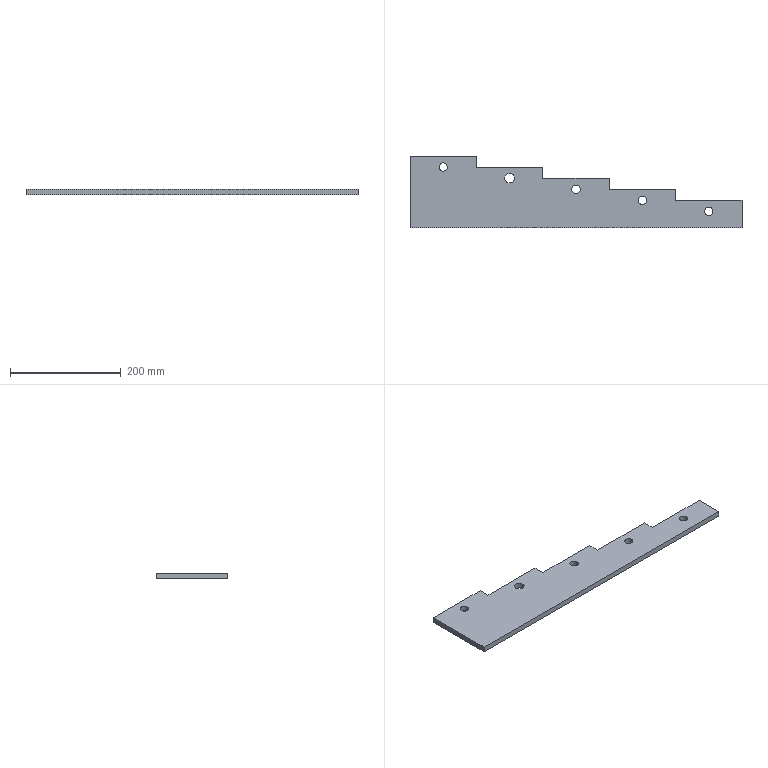Part | SolidWorks | features Extrusion 1 | 1 solid | 24 faces | box 600 x 130 x 10 mm | volume 530579 mm3 | plane 14 | cylinder 10 | commonest cylinder face diameters 15 x8 17.305 x2
STEP:
#1=CARTESIAN_POINT('',(532.5,30.,10.));
#2=VERTEX_POINT('',#1);
#3=CARTESIAN_POINT('',(547.5,30.,10.));
#4=VERTEX_POINT('',#3);
#5=CARTESIAN_POINT('',(540.,30.,10.));
#6=DIRECTION('',(0.,0.,1.));
#7=DIRECTION('',(1.,0.,0.));
#8=AXIS2_PLACEMENT_3D('',#5,#6,#7);
#9=CIRCLE('',#8,7.5);
#10=EDGE_CURVE('',#2,#4,#9,.T.);
#11=ORIENTED_EDGE('',*,*,#10,.T.);
#12=CARTESIAN_POINT('',(547.5,30.,0.));
#13=VERTEX_POINT('',#12);
#14=CARTESIAN_POINT('',(547.5,30.,10.));
#15=DIRECTION('',(0.,0.,-1.));
#16=VECTOR('',#15,1000.);
#17=LINE('',#14,#16);
#18=EDGE_CURVE('',#4,#13,#17,.T.);
#19=ORIENTED_EDGE('',*,*,#18,.T.);
#20=CARTESIAN_POINT('',(532.5,30.,0.));
#21=VERTEX_POINT('',#20);
#22=CARTESIAN_POINT('',(540.,30.,0.));
#23=DIRECTION('',(0.,0.,1.));
#24=DIRECTION('',(1.,0.,0.));
#25=AXIS2_PLACEMENT_3D('',#22,#23,#24);
#26=CIRCLE('',#25,7.5);
#27=EDGE_CURVE('',#21,#13,#26,.T.);
#28=ORIENTED_EDGE('',*,*,#27,.F.);
#29=CARTESIAN_POINT('',(532.5,30.,10.));
#30=DIRECTION('',(0.,0.,-1.));
#31=VECTOR('',#30,1000.);
#32=LINE('',#29,#31);
#33=EDGE_CURVE('',#2,#21,#32,.T.);
#34=ORIENTED_EDGE('',*,*,#33,.F.);
#35=EDGE_LOOP('',(#11,#19,#28,#34));
#36=FACE_OUTER_BOUND('',#35,.T.);
#37=CARTESIAN_POINT('',(540.,30.,10.));
#38=DIRECTION('',(0.,0.,-1.));
#39=DIRECTION('',(-1.,0.,0.));
#40=AXIS2_PLACEMENT_3D('',#37,#38,#39);
#41=CYLINDRICAL_SURFACE('',#40,7.5);
#42=ADVANCED_FACE('',(#36),#41,.F.);
#43=CARTESIAN_POINT('',(412.5,50.,10.));
#44=VERTEX_POINT('',#43);
#45=CARTESIAN_POINT('',(427.5,50.,10.));
#46=VERTEX_POINT('',#45);
#47=CARTESIAN_POINT('',(420.,50.,10.));
#48=DIRECTION('',(0.,0.,1.));
#49=DIRECTION('',(1.,0.,0.));
#50=AXIS2_PLACEMENT_3D('',#47,#48,#49);
#51=CIRCLE('',#50,7.5);
#52=EDGE_CURVE('',#44,#46,#51,.T.);
#53=ORIENTED_EDGE('',*,*,#52,.T.);
#54=CARTESIAN_POINT('',(427.5,50.,0.));
#55=VERTEX_POINT('',#54);
#56=CARTESIAN_POINT('',(427.5,50.,10.));
#57=DIRECTION('',(0.,0.,-1.));
#58=VECTOR('',#57,1000.);
#59=LINE('',#56,#58);
#60=EDGE_CURVE('',#46,#55,#59,.T.);
#61=ORIENTED_EDGE('',*,*,#60,.T.);
#62=CARTESIAN_POINT('',(412.5,50.,0.));
#63=VERTEX_POINT('',#62);
#64=CARTESIAN_POINT('',(420.,50.,0.));
#65=DIRECTION('',(0.,0.,1.));
#66=DIRECTION('',(1.,0.,0.));
#67=AXIS2_PLACEMENT_3D('',#64,#65,#66);
#68=CIRCLE('',#67,7.5);
#69=EDGE_CURVE('',#63,#55,#68,.T.);
#70=ORIENTED_EDGE('',*,*,#69,.F.);
#71=CARTESIAN_POINT('',(412.5,50.,10.));
#72=DIRECTION('',(0.,0.,-1.));
#73=VECTOR('',#72,1000.);
#74=LINE('',#71,#73);
#75=EDGE_CURVE('',#44,#63,#74,.T.);
#76=ORIENTED_EDGE('',*,*,#75,.F.);
#77=EDGE_LOOP('',(#53,#61,#70,#76));
#78=FACE_OUTER_BOUND('',#77,.T.);
#79=CARTESIAN_POINT('',(420.,50.,10.));
#80=DIRECTION('',(0.,0.,-1.));
#81=DIRECTION('',(-1.,0.,0.));
#82=AXIS2_PLACEMENT_3D('',#79,#80,#81);
#83=CYLINDRICAL_SURFACE('',#82,7.5);
#84=ADVANCED_FACE('',(#78),#83,.F.);
#85=CARTESIAN_POINT('',(292.5,70.,10.));
#86=VERTEX_POINT('',#85);
#87=CARTESIAN_POINT('',(307.5,70.,10.));
#88=VERTEX_POINT('',#87);
#89=CARTESIAN_POINT('',(300.,70.,10.));
#90=DIRECTION('',(0.,0.,1.));
#91=DIRECTION('',(1.,0.,0.));
#92=AXIS2_PLACEMENT_3D('',#89,#90,#91);
#93=CIRCLE('',#92,7.5);
#94=EDGE_CURVE('',#86,#88,#93,.T.);
#95=ORIENTED_EDGE('',*,*,#94,.T.);
#96=CARTESIAN_POINT('',(307.5,70.,0.));
#97=VERTEX_POINT('',#96);
#98=CARTESIAN_POINT('',(307.5,70.,10.));
#99=DIRECTION('',(0.,0.,-1.));
#100=VECTOR('',#99,1000.);
#101=LINE('',#98,#100);
#102=EDGE_CURVE('',#88,#97,#101,.T.);
#103=ORIENTED_EDGE('',*,*,#102,.T.);
#104=CARTESIAN_POINT('',(292.5,70.,0.));
#105=VERTEX_POINT('',#104);
#106=CARTESIAN_POINT('',(300.,70.,0.));
#107=DIRECTION('',(0.,0.,1.));
#108=DIRECTION('',(1.,0.,0.));
#109=AXIS2_PLACEMENT_3D('',#106,#107,#108);
#110=CIRCLE('',#109,7.5);
#111=EDGE_CURVE('',#105,#97,#110,.T.);
#112=ORIENTED_EDGE('',*,*,#111,.F.);
#113=CARTESIAN_POINT('',(292.5,70.,10.));
#114=DIRECTION('',(0.,0.,-1.));
#115=VECTOR('',#114,1000.);
#116=LINE('',#113,#115);
#117=EDGE_CURVE('',#86,#105,#116,.T.);
#118=ORIENTED_EDGE('',*,*,#117,.F.);
#119=EDGE_LOOP('',(#95,#103,#112,#118));
#120=FACE_OUTER_BOUND('',#119,.T.);
#121=CARTESIAN_POINT('',(300.,70.,10.));
#122=DIRECTION('',(0.,0.,-1.));
#123=DIRECTION('',(-1.,0.,0.));
#124=AXIS2_PLACEMENT_3D('',#121,#122,#123);
#125=CYLINDRICAL_SURFACE('',#124,7.5);
#126=ADVANCED_FACE('',(#120),#125,.F.);
#127=CARTESIAN_POINT('',(171.348,90.,10.));
#128=VERTEX_POINT('',#127);
#129=CARTESIAN_POINT('',(188.652,90.,10.));
#130=VERTEX_POINT('',#129);
#131=CARTESIAN_POINT('',(180.,90.,10.));
#132=DIRECTION('',(0.,0.,1.));
#133=DIRECTION('',(1.,0.,0.));
#134=AXIS2_PLACEMENT_3D('',#131,#132,#133);
#135=CIRCLE('',#134,8.652);
#136=EDGE_CURVE('',#128,#130,#135,.T.);
#137=ORIENTED_EDGE('',*,*,#136,.T.);
#138=CARTESIAN_POINT('',(188.652,90.,0.));
#139=VERTEX_POINT('',#138);
#140=CARTESIAN_POINT('',(188.652,90.,10.));
#141=DIRECTION('',(0.,0.,-1.));
#142=VECTOR('',#141,1000.);
#143=LINE('',#140,#142);
#144=EDGE_CURVE('',#130,#139,#143,.T.);
#145=ORIENTED_EDGE('',*,*,#144,.T.);
#146=CARTESIAN_POINT('',(171.348,90.,0.));
#147=VERTEX_POINT('',#146);
#148=CARTESIAN_POINT('',(180.,90.,0.));
#149=DIRECTION('',(0.,0.,1.));
#150=DIRECTION('',(1.,0.,0.));
#151=AXIS2_PLACEMENT_3D('',#148,#149,#150);
#152=CIRCLE('',#151,8.652);
#153=EDGE_CURVE('',#147,#139,#152,.T.);
#154=ORIENTED_EDGE('',*,*,#153,.F.);
#155=CARTESIAN_POINT('',(171.348,90.,10.));
#156=DIRECTION('',(0.,0.,-1.));
#157=VECTOR('',#156,1000.);
#158=LINE('',#155,#157);
#159=EDGE_CURVE('',#128,#147,#158,.T.);
#160=ORIENTED_EDGE('',*,*,#159,.F.);
#161=EDGE_LOOP('',(#137,#145,#154,#160));
#162=FACE_OUTER_BOUND('',#161,.T.);
#163=CARTESIAN_POINT('',(180.,90.,10.));
#164=DIRECTION('',(0.,0.,-1.));
#165=DIRECTION('',(-1.,0.,0.));
#166=AXIS2_PLACEMENT_3D('',#163,#164,#165);
#167=CYLINDRICAL_SURFACE('',#166,8.652);
#168=ADVANCED_FACE('',(#162),#167,.F.);
#169=CARTESIAN_POINT('',(52.5,110.,10.));
#170=VERTEX_POINT('',#169);
#171=CARTESIAN_POINT('',(67.5,110.,10.));
#172=VERTEX_POINT('',#171);
#173=CARTESIAN_POINT('',(60.,110.,10.));
#174=DIRECTION('',(0.,0.,1.));
#175=DIRECTION('',(1.,0.,0.));
#176=AXIS2_PLACEMENT_3D('',#173,#174,#175);
#177=CIRCLE('',#176,7.5);
#178=EDGE_CURVE('',#170,#172,#177,.T.);
#179=ORIENTED_EDGE('',*,*,#178,.T.);
#180=CARTESIAN_POINT('',(67.5,110.,0.));
#181=VERTEX_POINT('',#180);
#182=CARTESIAN_POINT('',(67.5,110.,10.));
#183=DIRECTION('',(0.,0.,-1.));
#184=VECTOR('',#183,1000.);
#185=LINE('',#182,#184);
#186=EDGE_CURVE('',#172,#181,#185,.T.);
#187=ORIENTED_EDGE('',*,*,#186,.T.);
#188=CARTESIAN_POINT('',(52.5,110.,0.));
#189=VERTEX_POINT('',#188);
#190=CARTESIAN_POINT('',(60.,110.,0.));
#191=DIRECTION('',(0.,0.,1.));
#192=DIRECTION('',(1.,0.,0.));
#193=AXIS2_PLACEMENT_3D('',#190,#191,#192);
#194=CIRCLE('',#193,7.5);
#195=EDGE_CURVE('',#189,#181,#194,.T.);
#196=ORIENTED_EDGE('',*,*,#195,.F.);
#197=CARTESIAN_POINT('',(52.5,110.,10.));
#198=DIRECTION('',(0.,0.,-1.));
#199=VECTOR('',#198,1000.);
#200=LINE('',#197,#199);
#201=EDGE_CURVE('',#170,#189,#200,.T.);
#202=ORIENTED_EDGE('',*,*,#201,.F.);
#203=EDGE_LOOP('',(#179,#187,#196,#202));
#204=FACE_OUTER_BOUND('',#203,.T.);
#205=CARTESIAN_POINT('',(60.,110.,10.));
#206=DIRECTION('',(0.,0.,-1.));
#207=DIRECTION('',(-1.,0.,0.));
#208=AXIS2_PLACEMENT_3D('',#205,#206,#207);
#209=CYLINDRICAL_SURFACE('',#208,7.5);
#210=ADVANCED_FACE('',(#204),#209,.F.);
#211=ORIENTED_EDGE('',*,*,#52,.F.);
#212=CARTESIAN_POINT('',(420.,50.,10.));
#213=DIRECTION('',(0.,0.,1.));
#214=DIRECTION('',(1.,0.,0.));
#215=AXIS2_PLACEMENT_3D('',#212,#213,#214);
#216=CIRCLE('',#215,7.5);
#217=EDGE_CURVE('',#46,#44,#216,.T.);
#218=ORIENTED_EDGE('',*,*,#217,.F.);
#219=EDGE_LOOP('',(#211,#218));
#220=FACE_BOUND('',#219,.T.);
#221=ORIENTED_EDGE('',*,*,#136,.F.);
#222=CARTESIAN_POINT('',(180.,90.,10.));
#223=DIRECTION('',(0.,0.,1.));
#224=DIRECTION('',(1.,0.,0.));
#225=AXIS2_PLACEMENT_3D('',#222,#223,#224);
#226=CIRCLE('',#225,8.652);
#227=EDGE_CURVE('',#130,#128,#226,.T.);
#228=ORIENTED_EDGE('',*,*,#227,.F.);
#229=EDGE_LOOP('',(#221,#228));
#230=FACE_BOUND('',#229,.T.);
#231=CARTESIAN_POINT('',(0.,130.,10.));
#232=VERTEX_POINT('',#231);
#233=CARTESIAN_POINT('',(0.,0.,10.));
#234=VERTEX_POINT('',#233);
#235=CARTESIAN_POINT('',(0.,130.,10.));
#236=DIRECTION('',(0.,-1.,0.));
#237=VECTOR('',#236,1000.);
#238=LINE('',#235,#237);
#239=EDGE_CURVE('',#232,#234,#238,.T.);
#240=ORIENTED_EDGE('',*,*,#239,.T.);
#241=CARTESIAN_POINT('',(600.,0.,10.));
#242=VERTEX_POINT('',#241);
#243=CARTESIAN_POINT('',(0.,0.,10.));
#244=DIRECTION('',(1.,0.,0.));
#245=VECTOR('',#244,1000.);
#246=LINE('',#243,#245);
#247=EDGE_CURVE('',#234,#242,#246,.T.);
#248=ORIENTED_EDGE('',*,*,#247,.T.);
#249=CARTESIAN_POINT('',(600.,50.,10.));
#250=VERTEX_POINT('',#249);
#251=CARTESIAN_POINT('',(600.,0.,10.));
#252=DIRECTION('',(0.,1.,0.));
#253=VECTOR('',#252,1000.);
#254=LINE('',#251,#253);
#255=EDGE_CURVE('',#242,#250,#254,.T.);
#256=ORIENTED_EDGE('',*,*,#255,.T.);
#257=CARTESIAN_POINT('',(480.,50.,10.));
#258=VERTEX_POINT('',#257);
#259=CARTESIAN_POINT('',(600.,50.,10.));
#260=DIRECTION('',(-1.,0.,0.));
#261=VECTOR('',#260,1000.);
#262=LINE('',#259,#261);
#263=EDGE_CURVE('',#250,#258,#262,.T.);
#264=ORIENTED_EDGE('',*,*,#263,.T.);
#265=CARTESIAN_POINT('',(480.,70.,10.));
#266=VERTEX_POINT('',#265);
#267=CARTESIAN_POINT('',(480.,50.,10.));
#268=DIRECTION('',(0.,1.,0.));
#269=VECTOR('',#268,1000.);
#270=LINE('',#267,#269);
#271=EDGE_CURVE('',#258,#266,#270,.T.);
#272=ORIENTED_EDGE('',*,*,#271,.T.);
#273=CARTESIAN_POINT('',(360.,70.,10.));
#274=VERTEX_POINT('',#273);
#275=CARTESIAN_POINT('',(480.,70.,10.));
#276=DIRECTION('',(-1.,0.,0.));
#277=VECTOR('',#276,1000.);
#278=LINE('',#275,#277);
#279=EDGE_CURVE('',#266,#274,#278,.T.);
#280=ORIENTED_EDGE('',*,*,#279,.T.);
#281=CARTESIAN_POINT('',(360.,90.,10.));
#282=VERTEX_POINT('',#281);
#283=CARTESIAN_POINT('',(360.,70.,10.));
#284=DIRECTION('',(0.,1.,0.));
#285=VECTOR('',#284,1000.);
#286=LINE('',#283,#285);
#287=EDGE_CURVE('',#274,#282,#286,.T.);
#288=ORIENTED_EDGE('',*,*,#287,.T.);
#289=CARTESIAN_POINT('',(240.,90.,10.));
#290=VERTEX_POINT('',#289);
#291=CARTESIAN_POINT('',(360.,90.,10.));
#292=DIRECTION('',(-1.,0.,0.));
#293=VECTOR('',#292,1000.);
#294=LINE('',#291,#293);
#295=EDGE_CURVE('',#282,#290,#294,.T.);
#296=ORIENTED_EDGE('',*,*,#295,.T.);
#297=CARTESIAN_POINT('',(240.,110.,10.));
#298=VERTEX_POINT('',#297);
#299=CARTESIAN_POINT('',(240.,90.,10.));
#300=DIRECTION('',(0.,1.,0.));
#301=VECTOR('',#300,1000.);
#302=LINE('',#299,#301);
#303=EDGE_CURVE('',#290,#298,#302,.T.);
#304=ORIENTED_EDGE('',*,*,#303,.T.);
#305=CARTESIAN_POINT('',(120.,110.,10.));
#306=VERTEX_POINT('',#305);
#307=CARTESIAN_POINT('',(240.,110.,10.));
#308=DIRECTION('',(-1.,0.,0.));
#309=VECTOR('',#308,1000.);
#310=LINE('',#307,#309);
#311=EDGE_CURVE('',#298,#306,#310,.T.);
#312=ORIENTED_EDGE('',*,*,#311,.T.);
#313=CARTESIAN_POINT('',(120.,130.,10.));
#314=VERTEX_POINT('',#313);
#315=CARTESIAN_POINT('',(120.,110.,10.));
#316=DIRECTION('',(0.,1.,0.));
#317=VECTOR('',#316,1000.);
#318=LINE('',#315,#317);
#319=EDGE_CURVE('',#306,#314,#318,.T.);
#320=ORIENTED_EDGE('',*,*,#319,.T.);
#321=CARTESIAN_POINT('',(120.,130.,10.));
#322=DIRECTION('',(-1.,0.,0.));
#323=VECTOR('',#322,1000.);
#324=LINE('',#321,#323);
#325=EDGE_CURVE('',#314,#232,#324,.T.);
#326=ORIENTED_EDGE('',*,*,#325,.T.);
#327=EDGE_LOOP('',(#240,#248,#256,#264,#272,#280,#288,#296,#304,#312,#320,#326));
#328=FACE_OUTER_BOUND('',#327,.T.);
#329=ORIENTED_EDGE('',*,*,#178,.F.);
#330=CARTESIAN_POINT('',(60.,110.,10.));
#331=DIRECTION('',(0.,0.,1.));
#332=DIRECTION('',(1.,0.,0.));
#333=AXIS2_PLACEMENT_3D('',#330,#331,#332);
#334=CIRCLE('',#333,7.5);
#335=EDGE_CURVE('',#172,#170,#334,.T.);
#336=ORIENTED_EDGE('',*,*,#335,.F.);
#337=EDGE_LOOP('',(#329,#336));
#338=FACE_BOUND('',#337,.T.);
#339=ORIENTED_EDGE('',*,*,#94,.F.);
#340=CARTESIAN_POINT('',(300.,70.,10.));
#341=DIRECTION('',(0.,0.,1.));
#342=DIRECTION('',(1.,0.,0.));
#343=AXIS2_PLACEMENT_3D('',#340,#341,#342);
#344=CIRCLE('',#343,7.5);
#345=EDGE_CURVE('',#88,#86,#344,.T.);
#346=ORIENTED_EDGE('',*,*,#345,.F.);
#347=EDGE_LOOP('',(#339,#346));
#348=FACE_BOUND('',#347,.T.);
#349=ORIENTED_EDGE('',*,*,#10,.F.);
#350=CARTESIAN_POINT('',(540.,30.,10.));
#351=DIRECTION('',(0.,0.,1.));
#352=DIRECTION('',(1.,0.,0.));
#353=AXIS2_PLACEMENT_3D('',#350,#351,#352);
#354=CIRCLE('',#353,7.5);
#355=EDGE_CURVE('',#4,#2,#354,.T.);
#356=ORIENTED_EDGE('',*,*,#355,.F.);
#357=EDGE_LOOP('',(#349,#356));
#358=FACE_BOUND('',#357,.T.);
#359=CARTESIAN_POINT('',(0.,0.,10.));
#360=DIRECTION('',(0.,0.,1.));
#361=DIRECTION('',(1.,0.,0.));
#362=AXIS2_PLACEMENT_3D('',#359,#360,#361);
#363=PLANE('',#362);
#364=ADVANCED_FACE('',(#220,#230,#328,#338,#348,#358),#363,.T.);
#365=CARTESIAN_POINT('',(0.,130.,0.));
#366=VERTEX_POINT('',#365);
#367=CARTESIAN_POINT('',(0.,0.,0.));
#368=VERTEX_POINT('',#367);
#369=CARTESIAN_POINT('',(0.,130.,0.));
#370=DIRECTION('',(0.,-1.,0.));
#371=VECTOR('',#370,1000.);
#372=LINE('',#369,#371);
#373=EDGE_CURVE('',#366,#368,#372,.T.);
#374=ORIENTED_EDGE('',*,*,#373,.F.);
#375=CARTESIAN_POINT('',(120.,130.,0.));
#376=VERTEX_POINT('',#375);
#377=CARTESIAN_POINT('',(120.,130.,0.));
#378=DIRECTION('',(-1.,0.,0.));
#379=VECTOR('',#378,1000.);
#380=LINE('',#377,#379);
#381=EDGE_CURVE('',#376,#366,#380,.T.);
#382=ORIENTED_EDGE('',*,*,#381,.F.);
#383=CARTESIAN_POINT('',(120.,110.,0.));
#384=VERTEX_POINT('',#383);
#385=CARTESIAN_POINT('',(120.,110.,0.));
#386=DIRECTION('',(0.,1.,0.));
#387=VECTOR('',#386,1000.);
#388=LINE('',#385,#387);
#389=EDGE_CURVE('',#384,#376,#388,.T.);
#390=ORIENTED_EDGE('',*,*,#389,.F.);
#391=CARTESIAN_POINT('',(240.,110.,0.));
#392=VERTEX_POINT('',#391);
#393=CARTESIAN_POINT('',(240.,110.,0.));
#394=DIRECTION('',(-1.,0.,0.));
#395=VECTOR('',#394,1000.);
#396=LINE('',#393,#395);
#397=EDGE_CURVE('',#392,#384,#396,.T.);
#398=ORIENTED_EDGE('',*,*,#397,.F.);
#399=CARTESIAN_POINT('',(240.,90.,0.));
#400=VERTEX_POINT('',#399);
#401=CARTESIAN_POINT('',(240.,90.,0.));
#402=DIRECTION('',(0.,1.,0.));
#403=VECTOR('',#402,1000.);
#404=LINE('',#401,#403);
#405=EDGE_CURVE('',#400,#392,#404,.T.);
#406=ORIENTED_EDGE('',*,*,#405,.F.);
#407=CARTESIAN_POINT('',(360.,90.,0.));
#408=VERTEX_POINT('',#407);
#409=CARTESIAN_POINT('',(360.,90.,0.));
#410=DIRECTION('',(-1.,0.,0.));
#411=VECTOR('',#410,1000.);
#412=LINE('',#409,#411);
#413=EDGE_CURVE('',#408,#400,#412,.T.);
#414=ORIENTED_EDGE('',*,*,#413,.F.);
#415=CARTESIAN_POINT('',(360.,70.,0.));
#416=VERTEX_POINT('',#415);
#417=CARTESIAN_POINT('',(360.,70.,0.));
#418=DIRECTION('',(0.,1.,0.));
#419=VECTOR('',#418,1000.);
#420=LINE('',#417,#419);
#421=EDGE_CURVE('',#416,#408,#420,.T.);
#422=ORIENTED_EDGE('',*,*,#421,.F.);
#423=CARTESIAN_POINT('',(480.,70.,0.));
#424=VERTEX_POINT('',#423);
#425=CARTESIAN_POINT('',(480.,70.,0.));
#426=DIRECTION('',(-1.,0.,0.));
#427=VECTOR('',#426,1000.);
#428=LINE('',#425,#427);
#429=EDGE_CURVE('',#424,#416,#428,.T.);
#430=ORIENTED_EDGE('',*,*,#429,.F.);
#431=CARTESIAN_POINT('',(480.,50.,0.));
#432=VERTEX_POINT('',#431);
#433=CARTESIAN_POINT('',(480.,50.,0.));
#434=DIRECTION('',(0.,1.,0.));
#435=VECTOR('',#434,1000.);
#436=LINE('',#433,#435);
#437=EDGE_CURVE('',#432,#424,#436,.T.);
#438=ORIENTED_EDGE('',*,*,#437,.F.);
#439=CARTESIAN_POINT('',(600.,50.,0.));
#440=VERTEX_POINT('',#439);
#441=CARTESIAN_POINT('',(600.,50.,0.));
#442=DIRECTION('',(-1.,0.,0.));
#443=VECTOR('',#442,1000.);
#444=LINE('',#441,#443);
#445=EDGE_CURVE('',#440,#432,#444,.T.);
#446=ORIENTED_EDGE('',*,*,#445,.F.);
#447=CARTESIAN_POINT('',(600.,0.,0.));
#448=VERTEX_POINT('',#447);
#449=CARTESIAN_POINT('',(600.,0.,0.));
#450=DIRECTION('',(0.,1.,0.));
#451=VECTOR('',#450,1000.);
#452=LINE('',#449,#451);
#453=EDGE_CURVE('',#448,#440,#452,.T.);
#454=ORIENTED_EDGE('',*,*,#453,.F.);
#455=CARTESIAN_POINT('',(0.,0.,0.));
#456=DIRECTION('',(1.,0.,0.));
#457=VECTOR('',#456,1000.);
#458=LINE('',#455,#457);
#459=EDGE_CURVE('',#368,#448,#458,.T.);
#460=ORIENTED_EDGE('',*,*,#459,.F.);
#461=EDGE_LOOP('',(#374,#382,#390,#398,#406,#414,#422,#430,#438,#446,#454,#460));
#462=FACE_OUTER_BOUND('',#461,.T.);
#463=ORIENTED_EDGE('',*,*,#195,.T.);
#464=CARTESIAN_POINT('',(60.,110.,0.));
#465=DIRECTION('',(0.,0.,1.));
#466=DIRECTION('',(1.,0.,0.));
#467=AXIS2_PLACEMENT_3D('',#464,#465,#466);
#468=CIRCLE('',#467,7.5);
#469=EDGE_CURVE('',#181,#189,#468,.T.);
#470=ORIENTED_EDGE('',*,*,#469,.T.);
#471=EDGE_LOOP('',(#463,#470));
#472=FACE_BOUND('',#471,.T.);
#473=ORIENTED_EDGE('',*,*,#153,.T.);
#474=CARTESIAN_POINT('',(180.,90.,0.));
#475=DIRECTION('',(0.,0.,1.));
#476=DIRECTION('',(1.,0.,0.));
#477=AXIS2_PLACEMENT_3D('',#474,#475,#476);
#478=CIRCLE('',#477,8.652);
#479=EDGE_CURVE('',#139,#147,#478,.T.);
#480=ORIENTED_EDGE('',*,*,#479,.T.);
#481=EDGE_LOOP('',(#473,#480));
#482=FACE_BOUND('',#481,.T.);
#483=ORIENTED_EDGE('',*,*,#111,.T.);
#484=CARTESIAN_POINT('',(300.,70.,0.));
#485=DIRECTION('',(0.,0.,1.));
#486=DIRECTION('',(1.,0.,0.));
#487=AXIS2_PLACEMENT_3D('',#484,#485,#486);
#488=CIRCLE('',#487,7.5);
#489=EDGE_CURVE('',#97,#105,#488,.T.);
#490=ORIENTED_EDGE('',*,*,#489,.T.);
#491=EDGE_LOOP('',(#483,#490));
#492=FACE_BOUND('',#491,.T.);
#493=ORIENTED_EDGE('',*,*,#69,.T.);
#494=CARTESIAN_POINT('',(420.,50.,0.));
#495=DIRECTION('',(0.,0.,1.));
#496=DIRECTION('',(1.,0.,0.));
#497=AXIS2_PLACEMENT_3D('',#494,#495,#496);
#498=CIRCLE('',#497,7.5);
#499=EDGE_CURVE('',#55,#63,#498,.T.);
#500=ORIENTED_EDGE('',*,*,#499,.T.);
#501=EDGE_LOOP('',(#493,#500));
#502=FACE_BOUND('',#501,.T.);
#503=ORIENTED_EDGE('',*,*,#27,.T.);
#504=CARTESIAN_POINT('',(540.,30.,0.));
#505=DIRECTION('',(0.,0.,1.));
#506=DIRECTION('',(1.,0.,0.));
#507=AXIS2_PLACEMENT_3D('',#504,#505,#506);
#508=CIRCLE('',#507,7.5);
#509=EDGE_CURVE('',#13,#21,#508,.T.);
#510=ORIENTED_EDGE('',*,*,#509,.T.);
#511=EDGE_LOOP('',(#503,#510));
#512=FACE_BOUND('',#511,.T.);
#513=CARTESIAN_POINT('',(0.,0.,0.));
#514=DIRECTION('',(0.,0.,1.));
#515=DIRECTION('',(1.,0.,0.));
#516=AXIS2_PLACEMENT_3D('',#513,#514,#515);
#517=PLANE('',#516);
#518=ADVANCED_FACE('',(#462,#472,#482,#492,#502,#512),#517,.F.);
#519=ORIENTED_EDGE('',*,*,#373,.T.);
#520=CARTESIAN_POINT('',(0.,0.,10.));
#521=DIRECTION('',(0.,0.,-1.));
#522=VECTOR('',#521,1000.);
#523=LINE('',#520,#522);
#524=EDGE_CURVE('',#234,#368,#523,.T.);
#525=ORIENTED_EDGE('',*,*,#524,.F.);
#526=ORIENTED_EDGE('',*,*,#239,.F.);
#527=CARTESIAN_POINT('',(0.,130.,10.));
#528=DIRECTION('',(0.,0.,-1.));
#529=VECTOR('',#528,1000.);
#530=LINE('',#527,#529);
#531=EDGE_CURVE('',#232,#366,#530,.T.);
#532=ORIENTED_EDGE('',*,*,#531,.T.);
#533=EDGE_LOOP('',(#519,#525,#526,#532));
#534=FACE_OUTER_BOUND('',#533,.T.);
#535=CARTESIAN_POINT('',(0.,130.,10.));
#536=DIRECTION('',(1.,0.,0.));
#537=DIRECTION('',(0.,0.,-1.));
#538=AXIS2_PLACEMENT_3D('',#535,#536,#537);
#539=PLANE('',#538);
#540=ADVANCED_FACE('',(#534),#539,.F.);
#541=ORIENTED_EDGE('',*,*,#459,.T.);
#542=CARTESIAN_POINT('',(600.,0.,10.));
#543=DIRECTION('',(0.,0.,-1.));
#544=VECTOR('',#543,1000.);
#545=LINE('',#542,#544);
#546=EDGE_CURVE('',#242,#448,#545,.T.);
#547=ORIENTED_EDGE('',*,*,#546,.F.);
#548=ORIENTED_EDGE('',*,*,#247,.F.);
#549=ORIENTED_EDGE('',*,*,#524,.T.);
#550=EDGE_LOOP('',(#541,#547,#548,#549));
#551=FACE_OUTER_BOUND('',#550,.T.);
#552=CARTESIAN_POINT('',(0.,0.,10.));
#553=DIRECTION('',(0.,1.,0.));
#554=DIRECTION('',(0.,0.,1.));
#555=AXIS2_PLACEMENT_3D('',#552,#553,#554);
#556=PLANE('',#555);
#557=ADVANCED_FACE('',(#551),#556,.F.);
#558=ORIENTED_EDGE('',*,*,#453,.T.);
#559=CARTESIAN_POINT('',(600.,50.,10.));
#560=DIRECTION('',(0.,0.,-1.));
#561=VECTOR('',#560,1000.);
#562=LINE('',#559,#561);
#563=EDGE_CURVE('',#250,#440,#562,.T.);
#564=ORIENTED_EDGE('',*,*,#563,.F.);
#565=ORIENTED_EDGE('',*,*,#255,.F.);
#566=ORIENTED_EDGE('',*,*,#546,.T.);
#567=EDGE_LOOP('',(#558,#564,#565,#566));
#568=FACE_OUTER_BOUND('',#567,.T.);
#569=CARTESIAN_POINT('',(600.,0.,10.));
#570=DIRECTION('',(-1.,0.,0.));
#571=DIRECTION('',(0.,0.,1.));
#572=AXIS2_PLACEMENT_3D('',#569,#570,#571);
#573=PLANE('',#572);
#574=ADVANCED_FACE('',(#568),#573,.F.);
#575=ORIENTED_EDGE('',*,*,#445,.T.);
#576=CARTESIAN_POINT('',(480.,50.,10.));
#577=DIRECTION('',(0.,0.,-1.));
#578=VECTOR('',#577,1000.);
#579=LINE('',#576,#578);
#580=EDGE_CURVE('',#258,#432,#579,.T.);
#581=ORIENTED_EDGE('',*,*,#580,.F.);
#582=ORIENTED_EDGE('',*,*,#263,.F.);
#583=ORIENTED_EDGE('',*,*,#563,.T.);
#584=EDGE_LOOP('',(#575,#581,#582,#583));
#585=FACE_OUTER_BOUND('',#584,.T.);
#586=CARTESIAN_POINT('',(600.,50.,10.));
#587=DIRECTION('',(0.,-1.,0.));
#588=DIRECTION('',(1.,0.,0.));
#589=AXIS2_PLACEMENT_3D('',#586,#587,#588);
#590=PLANE('',#589);
#591=ADVANCED_FACE('',(#585),#590,.F.);
#592=ORIENTED_EDGE('',*,*,#437,.T.);
#593=CARTESIAN_POINT('',(480.,70.,10.));
#594=DIRECTION('',(0.,0.,-1.));
#595=VECTOR('',#594,1000.);
#596=LINE('',#593,#595);
#597=EDGE_CURVE('',#266,#424,#596,.T.);
#598=ORIENTED_EDGE('',*,*,#597,.F.);
#599=ORIENTED_EDGE('',*,*,#271,.F.);
#600=ORIENTED_EDGE('',*,*,#580,.T.);
#601=EDGE_LOOP('',(#592,#598,#599,#600));
#602=FACE_OUTER_BOUND('',#601,.T.);
#603=CARTESIAN_POINT('',(480.,50.,10.));
#604=DIRECTION('',(-1.,0.,0.));
#605=DIRECTION('',(0.,0.,1.));
#606=AXIS2_PLACEMENT_3D('',#603,#604,#605);
#607=PLANE('',#606);
#608=ADVANCED_FACE('',(#602),#607,.F.);
#609=ORIENTED_EDGE('',*,*,#429,.T.);
#610=CARTESIAN_POINT('',(360.,70.,10.));
#611=DIRECTION('',(0.,0.,-1.));
#612=VECTOR('',#611,1000.);
#613=LINE('',#610,#612);
#614=EDGE_CURVE('',#274,#416,#613,.T.);
#615=ORIENTED_EDGE('',*,*,#614,.F.);
#616=ORIENTED_EDGE('',*,*,#279,.F.);
#617=ORIENTED_EDGE('',*,*,#597,.T.);
#618=EDGE_LOOP('',(#609,#615,#616,#617));
#619=FACE_OUTER_BOUND('',#618,.T.);
#620=CARTESIAN_POINT('',(480.,70.,10.));
#621=DIRECTION('',(0.,-1.,0.));
#622=DIRECTION('',(1.,0.,0.));
#623=AXIS2_PLACEMENT_3D('',#620,#621,#622);
#624=PLANE('',#623);
#625=ADVANCED_FACE('',(#619),#624,.F.);
#626=ORIENTED_EDGE('',*,*,#421,.T.);
#627=CARTESIAN_POINT('',(360.,90.,10.));
#628=DIRECTION('',(0.,0.,-1.));
#629=VECTOR('',#628,1000.);
#630=LINE('',#627,#629);
#631=EDGE_CURVE('',#282,#408,#630,.T.);
#632=ORIENTED_EDGE('',*,*,#631,.F.);
#633=ORIENTED_EDGE('',*,*,#287,.F.);
#634=ORIENTED_EDGE('',*,*,#614,.T.);
#635=EDGE_LOOP('',(#626,#632,#633,#634));
#636=FACE_OUTER_BOUND('',#635,.T.);
#637=CARTESIAN_POINT('',(360.,70.,10.));
#638=DIRECTION('',(-1.,0.,0.));
#639=DIRECTION('',(0.,0.,1.));
#640=AXIS2_PLACEMENT_3D('',#637,#638,#639);
#641=PLANE('',#640);
#642=ADVANCED_FACE('',(#636),#641,.F.);
#643=ORIENTED_EDGE('',*,*,#413,.T.);
#644=CARTESIAN_POINT('',(240.,90.,10.));
#645=DIRECTION('',(0.,0.,-1.));
#646=VECTOR('',#645,1000.);
#647=LINE('',#644,#646);
#648=EDGE_CURVE('',#290,#400,#647,.T.);
#649=ORIENTED_EDGE('',*,*,#648,.F.);
#650=ORIENTED_EDGE('',*,*,#295,.F.);
#651=ORIENTED_EDGE('',*,*,#631,.T.);
#652=EDGE_LOOP('',(#643,#649,#650,#651));
#653=FACE_OUTER_BOUND('',#652,.T.);
#654=CARTESIAN_POINT('',(360.,90.,10.));
#655=DIRECTION('',(0.,-1.,0.));
#656=DIRECTION('',(1.,0.,0.));
#657=AXIS2_PLACEMENT_3D('',#654,#655,#656);
#658=PLANE('',#657);
#659=ADVANCED_FACE('',(#653),#658,.F.);
#660=ORIENTED_EDGE('',*,*,#405,.T.);
#661=CARTESIAN_POINT('',(240.,110.,10.));
#662=DIRECTION('',(0.,0.,-1.));
#663=VECTOR('',#662,1000.);
#664=LINE('',#661,#663);
#665=EDGE_CURVE('',#298,#392,#664,.T.);
#666=ORIENTED_EDGE('',*,*,#665,.F.);
#667=ORIENTED_EDGE('',*,*,#303,.F.);
#668=ORIENTED_EDGE('',*,*,#648,.T.);
#669=EDGE_LOOP('',(#660,#666,#667,#668));
#670=FACE_OUTER_BOUND('',#669,.T.);
#671=CARTESIAN_POINT('',(240.,90.,10.));
#672=DIRECTION('',(-1.,0.,0.));
#673=DIRECTION('',(0.,0.,1.));
#674=AXIS2_PLACEMENT_3D('',#671,#672,#673);
#675=PLANE('',#674);
#676=ADVANCED_FACE('',(#670),#675,.F.);
#677=ORIENTED_EDGE('',*,*,#397,.T.);
#678=CARTESIAN_POINT('',(120.,110.,10.));
#679=DIRECTION('',(0.,0.,-1.));
#680=VECTOR('',#679,1000.);
#681=LINE('',#678,#680);
#682=EDGE_CURVE('',#306,#384,#681,.T.);
#683=ORIENTED_EDGE('',*,*,#682,.F.);
#684=ORIENTED_EDGE('',*,*,#311,.F.);
#685=ORIENTED_EDGE('',*,*,#665,.T.);
#686=EDGE_LOOP('',(#677,#683,#684,#685));
#687=FACE_OUTER_BOUND('',#686,.T.);
#688=CARTESIAN_POINT('',(240.,110.,10.));
#689=DIRECTION('',(0.,-1.,0.));
#690=DIRECTION('',(1.,0.,0.));
#691=AXIS2_PLACEMENT_3D('',#688,#689,#690);
#692=PLANE('',#691);
#693=ADVANCED_FACE('',(#687),#692,.F.);
#694=ORIENTED_EDGE('',*,*,#389,.T.);
#695=CARTESIAN_POINT('',(120.,130.,10.));
#696=DIRECTION('',(0.,0.,-1.));
#697=VECTOR('',#696,1000.);
#698=LINE('',#695,#697);
#699=EDGE_CURVE('',#314,#376,#698,.T.);
#700=ORIENTED_EDGE('',*,*,#699,.F.);
#701=ORIENTED_EDGE('',*,*,#319,.F.);
#702=ORIENTED_EDGE('',*,*,#682,.T.);
#703=EDGE_LOOP('',(#694,#700,#701,#702));
#704=FACE_OUTER_BOUND('',#703,.T.);
#705=CARTESIAN_POINT('',(120.,110.,10.));
#706=DIRECTION('',(-1.,0.,0.));
#707=DIRECTION('',(0.,0.,1.));
#708=AXIS2_PLACEMENT_3D('',#705,#706,#707);
#709=PLANE('',#708);
#710=ADVANCED_FACE('',(#704),#709,.F.);
#711=ORIENTED_EDGE('',*,*,#381,.T.);
#712=ORIENTED_EDGE('',*,*,#531,.F.);
#713=ORIENTED_EDGE('',*,*,#325,.F.);
#714=ORIENTED_EDGE('',*,*,#699,.T.);
#715=EDGE_LOOP('',(#711,#712,#713,#714));
#716=FACE_OUTER_BOUND('',#715,.T.);
#717=CARTESIAN_POINT('',(120.,130.,10.));
#718=DIRECTION('',(0.,-1.,0.));
#719=DIRECTION('',(1.,0.,0.));
#720=AXIS2_PLACEMENT_3D('',#717,#718,#719);
#721=PLANE('',#720);
#722=ADVANCED_FACE('',(#716),#721,.F.);
#723=ORIENTED_EDGE('',*,*,#186,.F.);
#724=ORIENTED_EDGE('',*,*,#335,.T.);
#725=ORIENTED_EDGE('',*,*,#201,.T.);
#726=ORIENTED_EDGE('',*,*,#469,.F.);
#727=EDGE_LOOP('',(#723,#724,#725,#726));
#728=FACE_OUTER_BOUND('',#727,.T.);
#729=CARTESIAN_POINT('',(60.,110.,10.));
#730=DIRECTION('',(0.,0.,-1.));
#731=DIRECTION('',(-1.,0.,0.));
#732=AXIS2_PLACEMENT_3D('',#729,#730,#731);
#733=CYLINDRICAL_SURFACE('',#732,7.5);
#734=ADVANCED_FACE('',(#728),#733,.F.);
#735=ORIENTED_EDGE('',*,*,#144,.F.);
#736=ORIENTED_EDGE('',*,*,#227,.T.);
#737=ORIENTED_EDGE('',*,*,#159,.T.);
#738=ORIENTED_EDGE('',*,*,#479,.F.);
#739=EDGE_LOOP('',(#735,#736,#737,#738));
#740=FACE_OUTER_BOUND('',#739,.T.);
#741=CARTESIAN_POINT('',(180.,90.,10.));
#742=DIRECTION('',(0.,0.,-1.));
#743=DIRECTION('',(-1.,0.,0.));
#744=AXIS2_PLACEMENT_3D('',#741,#742,#743);
#745=CYLINDRICAL_SURFACE('',#744,8.652);
#746=ADVANCED_FACE('',(#740),#745,.F.);
#747=ORIENTED_EDGE('',*,*,#102,.F.);
#748=ORIENTED_EDGE('',*,*,#345,.T.);
#749=ORIENTED_EDGE('',*,*,#117,.T.);
#750=ORIENTED_EDGE('',*,*,#489,.F.);
#751=EDGE_LOOP('',(#747,#748,#749,#750));
#752=FACE_OUTER_BOUND('',#751,.T.);
#753=CARTESIAN_POINT('',(300.,70.,10.));
#754=DIRECTION('',(0.,0.,-1.));
#755=DIRECTION('',(-1.,0.,0.));
#756=AXIS2_PLACEMENT_3D('',#753,#754,#755);
#757=CYLINDRICAL_SURFACE('',#756,7.5);
#758=ADVANCED_FACE('',(#752),#757,.F.);
#759=ORIENTED_EDGE('',*,*,#60,.F.);
#760=ORIENTED_EDGE('',*,*,#217,.T.);
#761=ORIENTED_EDGE('',*,*,#75,.T.);
#762=ORIENTED_EDGE('',*,*,#499,.F.);
#763=EDGE_LOOP('',(#759,#760,#761,#762));
#764=FACE_OUTER_BOUND('',#763,.T.);
#765=CARTESIAN_POINT('',(420.,50.,10.));
#766=DIRECTION('',(0.,0.,-1.));
#767=DIRECTION('',(-1.,0.,0.));
#768=AXIS2_PLACEMENT_3D('',#765,#766,#767);
#769=CYLINDRICAL_SURFACE('',#768,7.5);
#770=ADVANCED_FACE('',(#764),#769,.F.);
#771=ORIENTED_EDGE('',*,*,#18,.F.);
#772=ORIENTED_EDGE('',*,*,#355,.T.);
#773=ORIENTED_EDGE('',*,*,#33,.T.);
#774=ORIENTED_EDGE('',*,*,#509,.F.);
#775=EDGE_LOOP('',(#771,#772,#773,#774));
#776=FACE_OUTER_BOUND('',#775,.T.);
#777=CARTESIAN_POINT('',(540.,30.,10.));
#778=DIRECTION('',(0.,0.,-1.));
#779=DIRECTION('',(-1.,0.,0.));
#780=AXIS2_PLACEMENT_3D('',#777,#778,#779);
#781=CYLINDRICAL_SURFACE('',#780,7.5);
#782=ADVANCED_FACE('',(#776),#781,.F.);
#783=CLOSED_SHELL('',(#42,#84,#126,#168,#210,#364,#518,#540,#557,#574,#591,#608,#625,#642,#659,#676,#693,#710,#722,#734,#746,#758,#770,#782));
#784=MANIFOLD_SOLID_BREP('',#783);
#785=CARTESIAN_POINT('',(0.,0.,0.));
#786=DIRECTION('',(0.,0.,1.));
#787=DIRECTION('',(1.,0.,0.));
#788=AXIS2_PLACEMENT_3D('',#785,#786,#787);
#789=(LENGTH_UNIT()NAMED_UNIT(*)SI_UNIT(.MILLI.,.METRE.));
#790=UNCERTAINTY_MEASURE_WITH_UNIT(LENGTH_MEASURE(0.00001),#789,'','');
#791=(NAMED_UNIT(*)PLANE_ANGLE_UNIT()SI_UNIT($,.RADIAN.));
#792=(NAMED_UNIT(*)SI_UNIT($,.STERADIAN.)SOLID_ANGLE_UNIT());
#793=(GEOMETRIC_REPRESENTATION_CONTEXT(3)GLOBAL_UNCERTAINTY_ASSIGNED_CONTEXT((#790))GLOBAL_UNIT_ASSIGNED_CONTEXT((#789,#791,#792))REPRESENTATION_CONTEXT('',''));
#794=ADVANCED_BREP_SHAPE_REPRESENTATION('',(#784,#788),#793);